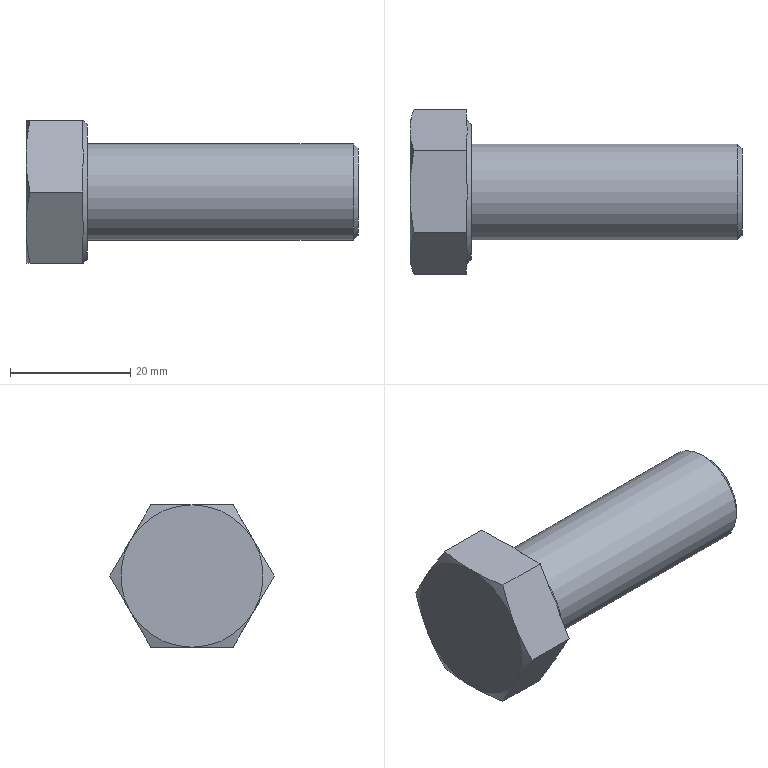Part | STEP file | Hex head bolt M16X45 A2-70 GBT5783-2016_GB_FASTENER_BOLT_STBAB A M16X45-N | 1 solid | 24 faces | box 55.18 x 27.332 x 23.67 mm | volume 13915 mm3 | plane 15 | cone 8 | cylinder 1 | commonest cylinder face diameters 16 x1